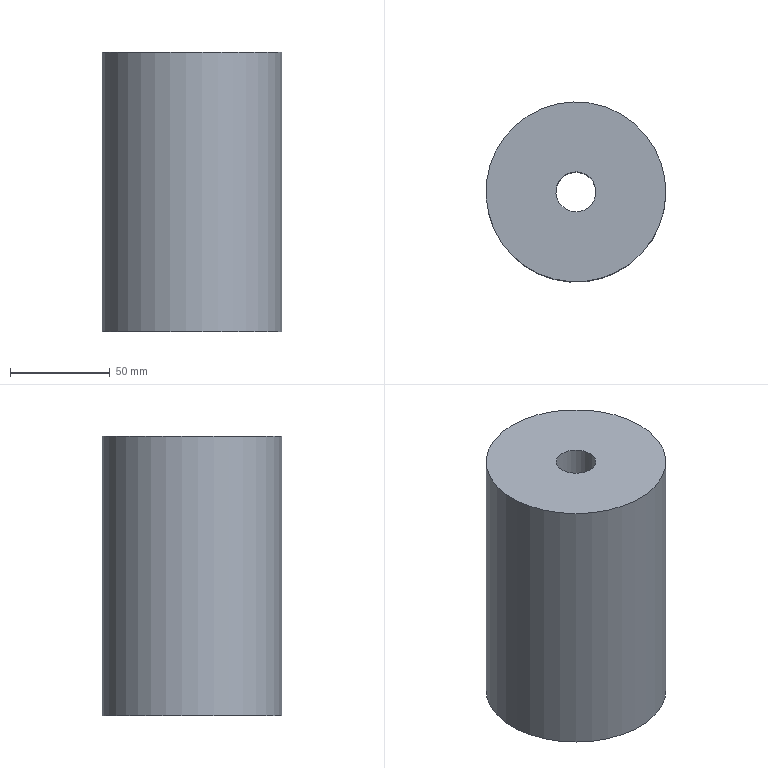Part | NX | features solid 2 | 1 solid | 4 faces | box 90 x 90 x 140 mm | volume 846659 mm3 | plane 2 | cylinder 2 | commonest cylinder face diameters 20 x1 90 x1
STEP:
#1=CARTESIAN_POINT('',(1433.632,829.14,10.));
#2=VERTEX_POINT('',#1);
#3=CARTESIAN_POINT('',(1465.452,860.96,10.));
#4=DIRECTION('',(0.,0.,1.));
#5=DIRECTION('',(-0.7071,-0.7071,0.));
#6=AXIS2_PLACEMENT_3D('',#3,#4,#5);
#7=CIRCLE('',#6,45.);
#8=EDGE_CURVE('',#2,#2,#7,.T.);
#9=ORIENTED_EDGE('',*,*,#8,.T.);
#10=EDGE_LOOP('',(#9));
#11=FACE_BOUND('',#10,.T.);
#12=CARTESIAN_POINT('',(1458.38,853.889,10.));
#13=VERTEX_POINT('',#12);
#14=CARTESIAN_POINT('',(1465.452,860.96,10.));
#15=DIRECTION('',(0.,0.,1.));
#16=DIRECTION('',(-0.7071,-0.7071,0.));
#17=AXIS2_PLACEMENT_3D('',#14,#15,#16);
#18=CIRCLE('',#17,10.);
#19=EDGE_CURVE('',#13,#13,#18,.T.);
#20=ORIENTED_EDGE('',*,*,#19,.F.);
#21=EDGE_LOOP('',(#20));
#22=FACE_BOUND('',#21,.T.);
#23=CARTESIAN_POINT('',(1465.452,860.96,10.));
#24=DIRECTION('',(0.,0.,-1.));
#25=DIRECTION('',(0.7071,0.7071,0.));
#26=AXIS2_PLACEMENT_3D('',#23,#24,#25);
#27=PLANE('',#26);
#28=ADVANCED_FACE('',(#11,#22),#27,.F.);
#29=CARTESIAN_POINT('',(1433.632,829.14,-130.));
#30=VERTEX_POINT('',#29);
#31=CARTESIAN_POINT('',(1465.452,860.96,-130.));
#32=DIRECTION('',(0.,0.,1.));
#33=DIRECTION('',(-0.7071,-0.7071,0.));
#34=AXIS2_PLACEMENT_3D('',#31,#32,#33);
#35=CIRCLE('',#34,45.);
#36=EDGE_CURVE('',#30,#30,#35,.T.);
#37=ORIENTED_EDGE('',*,*,#36,.F.);
#38=EDGE_LOOP('',(#37));
#39=FACE_BOUND('',#38,.T.);
#40=CARTESIAN_POINT('',(1458.38,853.889,-130.));
#41=VERTEX_POINT('',#40);
#42=CARTESIAN_POINT('',(1465.452,860.96,-130.));
#43=DIRECTION('',(0.,0.,1.));
#44=DIRECTION('',(-0.7071,-0.7071,0.));
#45=AXIS2_PLACEMENT_3D('',#42,#43,#44);
#46=CIRCLE('',#45,10.);
#47=EDGE_CURVE('',#41,#41,#46,.T.);
#48=ORIENTED_EDGE('',*,*,#47,.T.);
#49=EDGE_LOOP('',(#48));
#50=FACE_BOUND('',#49,.T.);
#51=CARTESIAN_POINT('',(1465.452,860.96,-130.));
#52=DIRECTION('',(0.,0.,-1.));
#53=DIRECTION('',(0.7071,0.7071,0.));
#54=AXIS2_PLACEMENT_3D('',#51,#52,#53);
#55=PLANE('',#54);
#56=ADVANCED_FACE('',(#39,#50),#55,.T.);
#57=ORIENTED_EDGE('',*,*,#8,.F.);
#58=EDGE_LOOP('',(#57));
#59=FACE_BOUND('',#58,.T.);
#60=ORIENTED_EDGE('',*,*,#36,.T.);
#61=EDGE_LOOP('',(#60));
#62=FACE_BOUND('',#61,.T.);
#63=CARTESIAN_POINT('',(1465.452,860.96,-130.));
#64=DIRECTION('',(0.,0.,1.));
#65=DIRECTION('',(-0.7071,-0.7071,0.));
#66=AXIS2_PLACEMENT_3D('',#63,#64,#65);
#67=CYLINDRICAL_SURFACE('',#66,45.);
#68=ADVANCED_FACE('',(#59,#62),#67,.T.);
#69=ORIENTED_EDGE('',*,*,#19,.T.);
#70=EDGE_LOOP('',(#69));
#71=FACE_BOUND('',#70,.T.);
#72=ORIENTED_EDGE('',*,*,#47,.F.);
#73=EDGE_LOOP('',(#72));
#74=FACE_BOUND('',#73,.T.);
#75=CARTESIAN_POINT('',(1465.452,860.96,-130.));
#76=DIRECTION('',(0.,0.,1.));
#77=DIRECTION('',(-0.7071,-0.7071,0.));
#78=AXIS2_PLACEMENT_3D('',#75,#76,#77);
#79=CYLINDRICAL_SURFACE('',#78,10.);
#80=ADVANCED_FACE('',(#71,#74),#79,.F.);
#81=CLOSED_SHELL('',(#28,#56,#68,#80));
#82=MANIFOLD_SOLID_BREP('',#81);
#83=(LENGTH_UNIT()NAMED_UNIT(*)SI_UNIT(.MILLI.,.METRE.));
#84=UNCERTAINTY_MEASURE_WITH_UNIT(LENGTH_MEASURE(0.00001),#83,'','');
#85=(NAMED_UNIT(*)PLANE_ANGLE_UNIT()SI_UNIT($,.RADIAN.));
#86=(NAMED_UNIT(*)SI_UNIT($,.STERADIAN.)SOLID_ANGLE_UNIT());
#87=(GEOMETRIC_REPRESENTATION_CONTEXT(3)GLOBAL_UNCERTAINTY_ASSIGNED_CONTEXT((#84))GLOBAL_UNIT_ASSIGNED_CONTEXT((#83,#85,#86))REPRESENTATION_CONTEXT('',''));
#88=ADVANCED_BREP_SHAPE_REPRESENTATION('',(#82),#87);